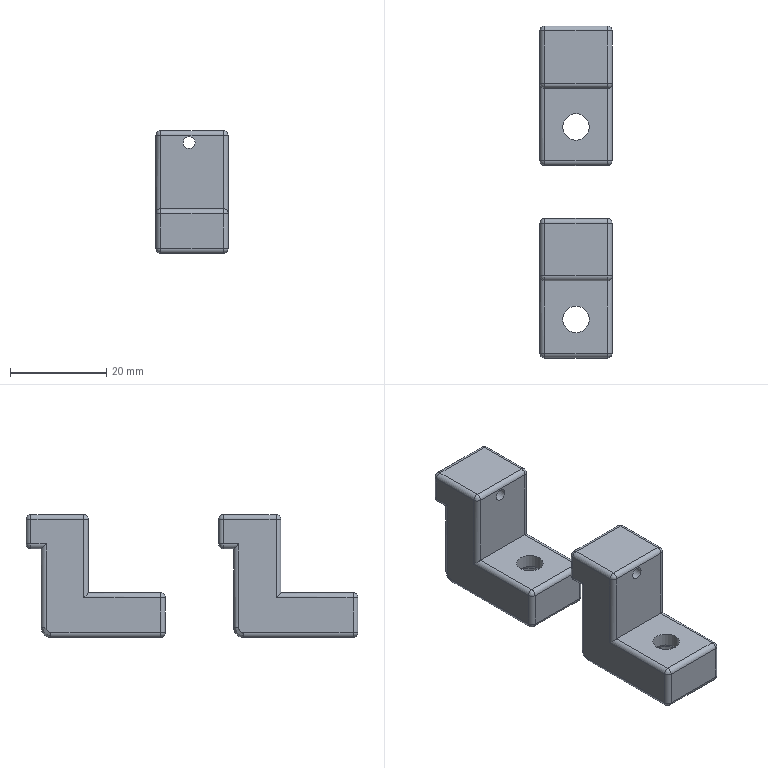Part | 2 solids | 98 faces | box 15 x 68.95 x 25.5 mm | volume 11252 mm3 | cylinder 50 | plane 22 | sphere 20 | spline 4 | cone 2 | commonest cylinder face diameters 2 x42 2.5 x2 4 x2 5.5 x2 10 x2